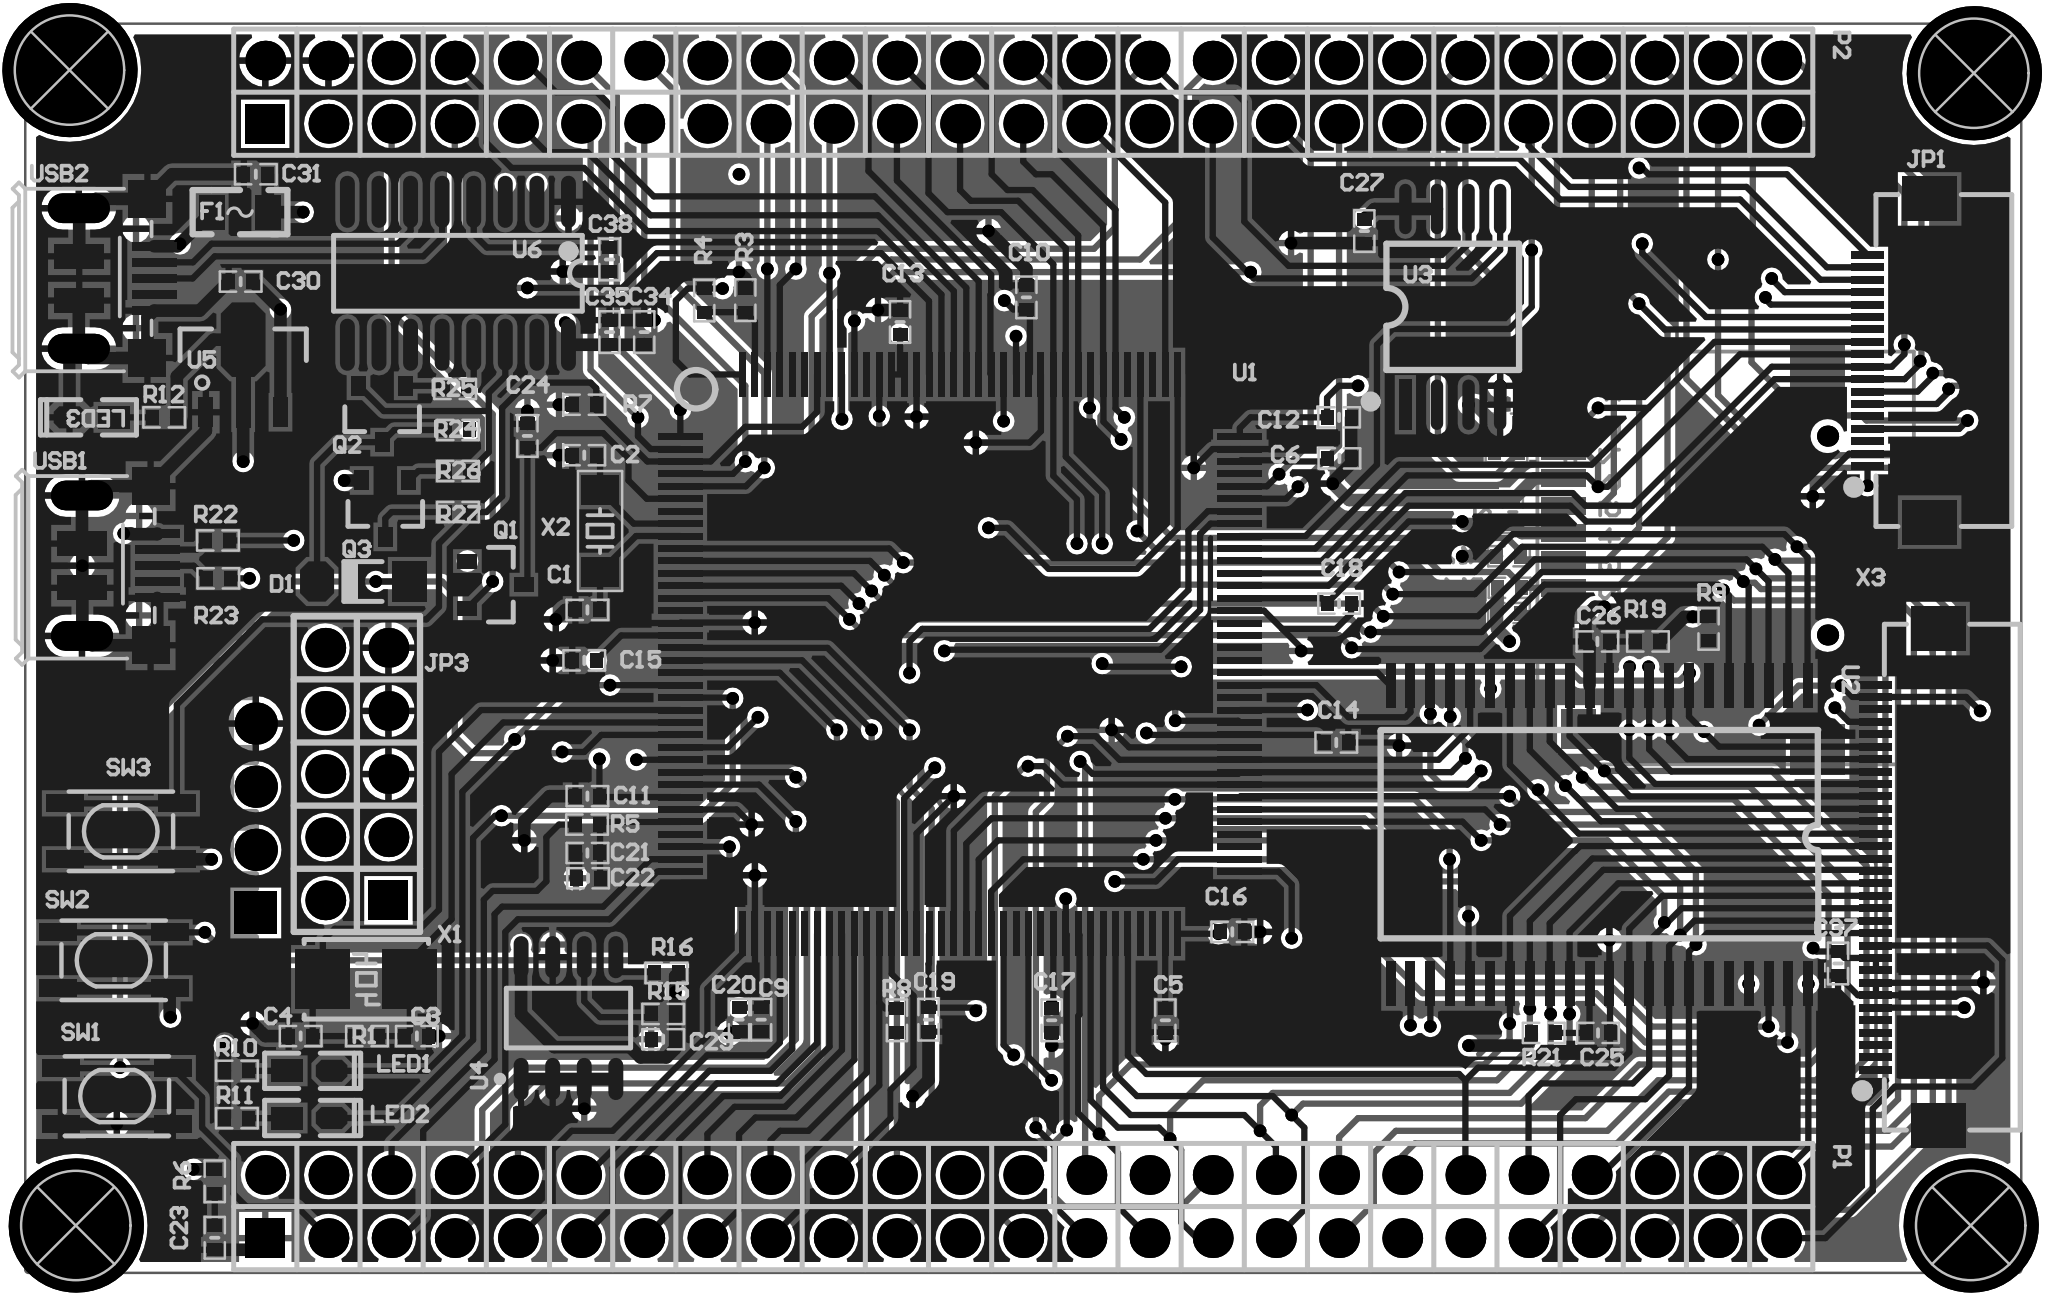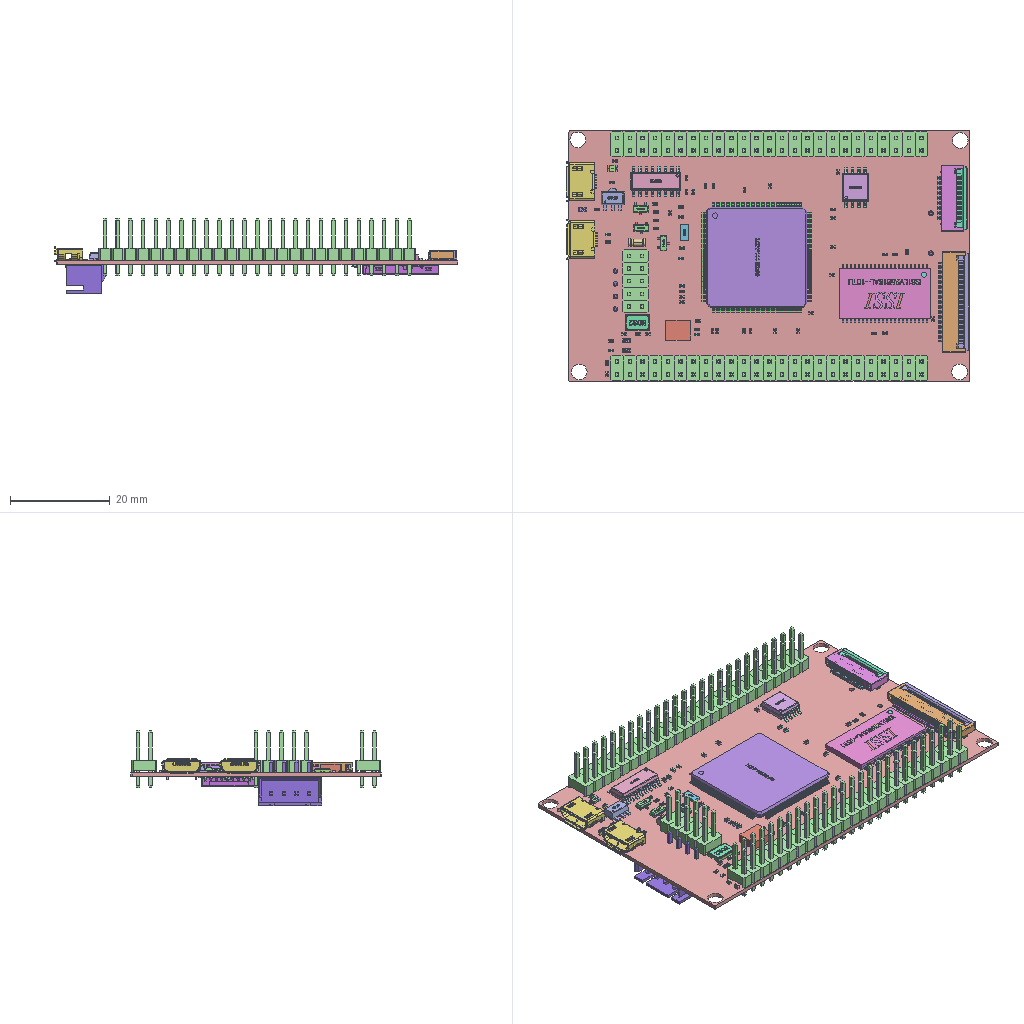Circuit board layout | Altium Designer | box 80.8 x 50.3 x 15 mm
Layer stack:
# Altium Designer layer stack of  (unit mm; dielectric type: 0 none, 1 core, 2 prepreg, 3 surface material)
index,name,kind,layer,copper_thickness_mm,dielectric_type,dielectric_thickness_mm,dielectric_material,dielectric_constant
0,Top Paste,other,,,,,,
1,Top Overlay,other,,,,,,
2,Top Solder,dielectric,,,3,0.0102,Solder Resist,3.5
3,Top Layer,copper,Top Layer,0.0356,,,,
4,Dielectric 1,dielectric,,,1,0.254,FR-4,4.2
5,2,copper,2,0.036,,,,
6,Dielectric 4,dielectric,,,2,0.127,,4.2
7,VCC,copper,VCC,0.036,,,,
8,Dielectric 3,dielectric,,,1,0.254,,4.2
9,Bottom Layer,copper,Bottom Layer,0.0356,,,,
10,Bottom Solder,dielectric,,,3,0.0102,Solder Resist,3.5
11,Bottom Overlay,other,,,,,,
12,Bottom Paste,other,,,,,,
# drill layer pairs: low layer,high layer
drill_pair,Top Layer,Bottom Layer
Part placement:
Designator,Comment,Layer,Footprint,Center-X(mm),Center-Y(mm),Rotation
C1,10P,TopLayer,C_0402,47.879,51.943,0
C2,10P,TopLayer,C_0402,47.752,58.166,0
C3,22P,TopLayer,C_0402,41.021,34.798,180
C4,22P,TopLayer,C_0402,36.347,34.798,0
C5,225,TopLayer,C_0402,71.12,35.433,270
C6,225,TopLayer,C_0402,78.12,58.039,0
C9,104,TopLayer,C_0402,54.864,35.458,90
C10,104,TopLayer,C_0402,65.532,64.516,270
C11,104,TopLayer,C_0402,47.879,44.45,0
C12,104,TopLayer,C_0402,78.105,59.69,180
C13,104,TopLayer,C_0402,60.452,63.525,270
C14,104,TopLayer,C_0402,77.993,46.609,180
C15,104,TopLayer,C_0402,47.752,49.911,360
C16,104,TopLayer,C_0402,73.812,38.989,180
C17,104,TopLayer,C_0402,66.548,35.433,90
C18,104,TopLayer,C_0402,78.105,52.197,180
C19,104,TopLayer,C_0402,61.595,35.458,90
C20,104,TopLayer,C_0402,53.975,35.458,90
C21,10UF,TopLayer,C_0402,47.879,42.164,180
C22,104,TopLayer,C_0402,47.904,41.148,180
C23,104,TopLayer,C_0402,32.893,26.685,270
C24,104,TopLayer,C_0402,45.466,58.943,270
C25,10U,TopLayer,C_0402,88.519,34.925,360
C26,10U,TopLayer,C_0402,88.494,50.673,180
C27,104,TopLayer,C_0402,79.121,67.183,270
C28,104,BottomLayer,C_0402,85.09,55.88,270
C29,104,TopLayer,C_0402,50.927,34.671,360
C30,22UF,TopLayer,C_0402,33.934,65.151,360
C31,104,TopLayer,C_0402,34.544,69.469,360
C34,10UF,TopLayer,C_0402,50.165,63.119,90
C35,104,TopLayer,C_0402,48.768,63.119,90
C37,104,TopLayer,C_0402,98.171,37.719,90
C38,104,TopLayer,C_0402,48.768,66.04,90
D1,1N4148,TopLayer,MINI_MELF_(LL34),38.862,53.086,180
F1,MSMD200-8V 2A,TopLayer,FU_0805,33.909,67.945,0
HOLE1,M3,TopLayer,M3_5.4MM,103.505,27.178,0
HOLE2,M3,TopLayer,M3_5.4MM,27.305,27.178,0
HOLE3,M3,TopLayer,M3_5.4MM,27.051,73.66,0
HOLE4,M3,TopLayer,M3_5.4MM,103.632,73.533,0
J1,TF_Card,BottomLayer,Micro_SD,92.436,54.084,270
JP1,FPC0.5-18P,TopLayer,FPC0.5_2H-WS-18P,100.606,61.976,90
JP2,SWD,BottomLayer,XH2.54-WI-4P,34.544,43.561,90
JP3,Header 5X2,TopLayer,HDR2.54-LI-2x5P,38.608,45.339,90
LED1,Red,TopLayer,LED_0603R,36.703,33.401,360
LED2,Red,TopLayer,LED_0603R,36.703,31.503,360
LED3,Red,TopLayer,LED_0603R,27.94,59.69,180
P1,Header 25X2,TopLayer,HDR2.54-LI-2x25P,65.405,27.94,360
P2,Header 25X2,TopLayer,HDR2.54-LI-2x25P,65.405,72.771,360
Q1,BAT54C,TopLayer,SOT23-3L,44.187,52.959,270
Q2,SS8050,TopLayer,SOT23-3L,39.624,59.826,180
Q3,SS8550,TopLayer,SOT23-3L,39.751,56.016,180
R1,1M,TopLayer,R_0402,39.014,34.798,180
R3,0R,TopLayer,R_0402,54.229,64.404,90
R4,0R,TopLayer,R_0402,52.578,64.389,90
R5,10R,TopLayer,R_0402,47.864,43.307,0
R6,10K,TopLayer,R_0402,32.893,28.956,90
R7,10K,TopLayer,R_0402,47.752,60.198,0
R8,10K,TopLayer,R_0402,60.325,35.433,90
R9,10K,TopLayer,R_0402,92.964,51.181,90
R10,510,TopLayer,R_0402,33.782,33.401,180
R11,510,TopLayer,R_0402,33.782,31.496,180
R12,1K,TopLayer,R_0402,30.861,59.69,360
R13,47K,BottomLayer,R_0402,84.938,51.816,360
R14,47K,BottomLayer,R_0402,84.963,52.832,360
R15,4.7K,TopLayer,R_0402,50.927,35.687,360
R16,4.7K,TopLayer,R_0402,51.054,37.338,360
R17,47K,BottomLayer,R_0402,84.938,54.102,360
R18,47K,BottomLayer,R_0402,84.836,58.293,360
R19,2R,TopLayer,R_0402,90.526,50.673,180
R20,47K,BottomLayer,R_0402,84.836,59.436,360
R21,2R,TopLayer,R_0402,86.335,34.925,360
R22,10R,TopLayer,R_0402,33.02,54.737,360
R23,10R,TopLayer,R_0402,33.035,53.213,360
R24,10K,TopLayer,R_0402,42.672,59.182,180
R25,1K,TopLayer,R_0402,42.56,60.833,180
R26,1K,TopLayer,R_0402,42.672,57.531,180
R27,1K,TopLayer,R_0402,42.672,55.88,360
SW1,3x6x5,TopLayer,TSW_SMD-3*4*2.5,28.956,32.385,360
SW2,3x6x5,TopLayer,TSW_SMD-3*4*2.5,28.829,37.846,180
SW3,3x6x5,TopLayer,TSW_SMD-3*4*2.5,29.119,43.035,180
U1,STM32F407,TopLayer,LQFP144_20X20_M,62.865,50.165,270
U2,IS61LV51216,TopLayer,TSOP44_M,88.576,42.895,270
U3,W25Q128,TopLayer,SOP8W_L,82.677,64.135,90
U4,24C02C-E/ST,TopLayer,SOP8_L,47.117,35.523,90
U5,AS1117B,TopLayer,SOT89_L,34.036,61.355,0
U6,CH340G,TopLayer,SOP16,42.672,65.486,270
USB1,USB-DEVICE,TopLayer,USB-MICRO_B,29.067,53.721,270
USB2,USB-DEVICE,TopLayer,USB-MICRO_B,28.94,65.278,270
X1,8MHz,TopLayer,OSC_5032-2P,38.989,37.084,180
X2,32.768KHZ,TopLayer,OSC_3215-2P,48.387,55.118,270
X3,FPC0.5-32P,TopLayer,FPC0.5_2H-WS-32P,100.944,41.192,90
Pad and via stacks:
# Altium Designer via and pad stacks of  (unit mm). Each distinct definition once, with the count of objects using it.
# via: kind,start_layer,end_layer,hole_mm,diameter_mm,mode(0 simple;1 top-mid-bottom;2 full stack),diameter_per_layer,count,example_net
# pad: kind,layer,hole_mm,hole_type(0 round;1 square;2 slot),plating,top_size,top_shape(1 round;2 rect;3 octagon;9 rounded rect),mid_size,bottom_size,mode,footprint,size_per_layer,count,example
pad,Top Layer,0,0,plated,0.508x0.6,2,0.508x0.6,0.508x0.6,0,R 0402,,42,R27.2
pad,Top Layer,0,0,unplated,2.4x2.2,2,2.4x2.2,2.4x2.2,0,OSC 5032-2P,,2,X1.2
pad,Top Layer,0,0,plated,1.27x0.889,3,1.27x0.889,1.27x0.889,0,LED 0603R,,3,LED3.2
pad,Top Layer,0,0,plated,1.27x0.889,2,1.27x0.889,1.27x0.889,0,LED 0603R,,3,LED3.1
pad,Top Layer,0,0,plated,0.508x0.6,2,0.508x0.6,0.508x0.6,0,C 0402,,64,C38.2
pad,Top Layer,0,0,plated,1.62x1.37,2,1.62x1.37,1.62x1.37,0,MINI_MELF (LL34),,1,D1.1
pad,Top Layer,0,0,plated,1.62x1.37,3,1.62x1.37,1.62x1.37,0,MINI_MELF (LL34),,1,D1.2
pad,Top Layer,0,0,plated,1.016x1.397,2,1.016x1.397,1.016x1.397,0,FU 0805,,2,F1.1
pad,Top Layer,0,0,plated,0.6x0.8,2,0.6x0.8,0.6x0.8,0,SOT23-3L,,9,Q1.1
pad,Top Layer,0,0,plated,0.254x1.8,2,0.254x1.8,0.254x1.8,0,LQFP144 20X20_M,,144,U1.11
pad,Top Layer,0,0,plated,1.8x0.4,2,1.8x0.4,1.8x0.4,0,TSOP44_M,,44,U2.39
pad,Top Layer,0,0,plated,2.032x0.5,1,2.032x0.5,2.032x0.5,0,SOP8W_L,,7,U3.8
pad,Top Layer,0,0,plated,2.032x0.5,2,2.032x0.5,2.032x0.5,0,SOP8W_L,,1,U3.1
pad,Top Layer,0,0,plated,0.6x1.7,1,0.6x1.7,0.6x1.7,0,SOP8_L,,8,U4.5
pad,Top Layer,0,0,plated,1.8x3,3,1.8x3,1.8x3,0,SOT89_L,,1,U5.2
pad,Top Layer,0,0,plated,0.6x1.2,2,0.6x1.2,0.6x1.2,0,SOT89_L,,2,U5.3
pad,Top Layer,0,0,plated,0.6x2.1,2,0.6x2.1,0.6x2.1,0,SOT89_L,,1,U5.2
pad,Top Layer,0,0,plated,0.6x2.1,1,0.6x2.1,0.6x2.1,0,SOP16,,16,U6.9
pad,Top Layer,0,0,plated,0.35x1.8,2,0.35x1.8,0.35x1.8,0,USB-MICRO_B,,10,USB1.5
pad,Top Layer,0,0,plated,1x2,2,1x2,1x2,0,USB-MICRO_B,,4,USB1.5
pad,Top Layer,0,0,plated,1.5x1.5,2,1.5x1.5,1.5x1.5,0,USB-MICRO_B,,4,USB1.5
pad,Top Layer,0,0,plated,1.2x1.5,2,1.2x1.5,1.2x1.5,0,OSC 3215-2P,,2,X2.2
pad,Top Layer,0,0,plated,1.3x0.3,2,1.3x0.3,1.3x0.3,0,FPC0.5 2H-WS-32P,,32,X3.32
pad,Top Layer,0,0,plated,2.2x1.8,2,2.2x1.8,2.2x1.8,0,FPC0.5 2H-WS-32P,,2,X3.0
pad,Top Layer,0,0,plated,1.5x0.7,2,1.5x0.7,1.5x0.7,0,TSW SMD-3*4*2.5,,12,SW1.2
pad,Top Layer,0,0,plated,2.2x1.8,2,2.2x1.8,2.2x1.8,0,FPC0.5 2H-WS-18P,,2,JP1.0
pad,Top Layer,0,0,plated,1.3x0.3,2,1.3x0.3,1.3x0.3,0,FPC0.5 2H-WS-18P,,18,JP1.9
pad,Multi-Layer,1,0,unplated,0.85x0.85,1,0.85x0.85,0.85x0.85,0,Micro SD,,2,J1.0
pad,Multi-Layer,3.175,0,plated,5.4x5.4,1,5.4x5.4,5.4x5.4,0,M3 5.4MM,,4,HOLE1.0
pad,Multi-Layer,0.9,0,plated,1.6x1.6,1,1.6x1.6,1.6x1.6,0,HDR2.54-LI-2x5P,,9,JP3.10
pad,Multi-Layer,0.9,0,plated,1.6x1.6,2,1.6x1.6,1.6x1.6,0,HDR2.54-LI-2x5P,,1,JP3.1
pad,Multi-Layer,0.9,0,plated,1.6x1.6,2,1.6x1.6,1.6x1.6,0,HDR2.54-LI-2x25P,,2,P1.1
pad,Multi-Layer,0.9,0,plated,1.6x1.6,1,1.6x1.6,1.6x1.6,0,HDR2.54-LI-2x25P,,98,P1.2
pad,Multi-Layer,0.45,2,plated,2.5x1.2,1,2.5x1.2,2.5x1.2,0,USB-MICRO_B,,4,USB1.5
pad,Multi-Layer,0.6,0,unplated,0x0,1,0x0,0x0,0,USB-MICRO_B,,4,USB1.5
pad,Multi-Layer,0.9,0,plated,1.7x1.7,1,1.7x1.7,1.7x1.7,0,XH2.54-WI-4P,,3,JP2.4
pad,Multi-Layer,0.9,0,plated,1.7x1.7,2,1.7x1.7,1.7x1.7,0,XH2.54-WI-4P,,1,JP2.1
pad,Bottom Layer,0,0,plated,0.508x0.6,2,0.508x0.6,0.508x0.6,0,R 0402,,10,R17.2
pad,Bottom Layer,0,0,plated,0.508x0.6,2,0.508x0.6,0.508x0.6,0,C 0402,,2,C28.2
pad,Bottom Layer,0,0,plated,2.032x2.2,2,2.032x2.2,2.032x2.2,0,Micro SD,,2,J1.10
pad,Bottom Layer,0,0,plated,1.6x1.4,2,1.6x1.4,1.6x1.4,0,Micro SD,,1,J1.10
pad,Bottom Layer,0,0,plated,1.2x1.4,2,1.2x1.4,1.2x1.4,0,Micro SD,,1,J1.10
pad,Bottom Layer,0,0,plated,0.7x1.8,2,0.7x1.8,0.7x1.8,0,Micro SD,,9,J1.1
via,Top Layer,Bottom Layer,0.254,0.508,0,,216,GND
Copper pours:
name,layer,net,type(0 solid;1 hatched;2 none)
D,Top Layer,GND,0
D,Bottom Layer,GND,0
Design rules, without the lines most boards share:
# Altium Designer design rules of  (exported by Altium Designer, unit mm)
# columns: name | kind | enabled | priority | scope1 | scope2 | descriptor | typed fields (field=value)
Clearance | 0 | enabled | 1 | All | All | Clearance Constraint (Gap=7mil) (All),(All) | gap=0.1778
PlaneConnect | 6 | enabled | 1 | All | All | Power Plane Connect Rule(Relief Connect )(Expansion=20mil) (Conductor Width=10mil) (Air Gap=10mil) (Entries=4) (All) | relief_conductor_width=0.254 relief_entries=4 relief_expansion=0.508
PolygonConnect | 20 | enabled | 1 | All | All | Polygon Connect Rule(Relief Connect )(Conductor Width=10mil) (Relief Angle=90 Angle) (Entries=4) (Air Gap Width=10mil) (All),(All) | connect_style(0=relief,1=direct,2=none)=0 relief_conductor_width=0.254 relief_entries=4
Width | 2 | enabled | 1 | All | All | Width Constraint (Min=7mil) (Max=30mil) (Preferred=7mil) (All) |
RoutingVias | 11 | enabled | 1 | All | All | Routing Via (MinHoleWidth=28mil) (MaxHoleWidth=28mil) (PreferredHoleWidth=28mil) (MinWidth=50mil) (MaxWidth=50mil) (PreferedWidth=50mil) (All) | via_min_hole=0.7112 via_max_hole=0.7112 via_preferred_diameter=1.27 via_preferred_hole=0.7112
SolderMaskExpansion | 13 | enabled | 1 | All | All | Solder Mask Expansion (Expansion =4mil) (All) | expansion=0.1016
HoleSize | 42 | enabled | 1 | All | All | Hole Size Constraint (Min=1mil) (Max=99999mil) (All) |
DiffPairsRouting | 51 | enabled | 1 | All | All | Differential Pairs Uncoupled Length using the Gap Constraints (Min=10mil) (Max=10mil) (Prefered=10mil)  and Width Constraints (Min=15mil) (Max=15mil) (Prefered=15mil) (All) |
HoleToHoleClearance | 52 | enabled | 1 | All | All | Hole To Hole Clearance (Gap=10mil) (All),(All) | gap=0.254
MinimumSolderMaskSliver | 53 | enabled | 1 | All | All | Minimum Solder Mask Sliver (Gap=0mil) (All),(All) |
SilkToSolderMaskClearance | 54 | enabled | 1 | IsPad | All | Silk To Solder Mask (Clearance=0mil) (IsPad),(All) |
SilkToSilkClearance | 55 | enabled | 1 | All | All | Silk to Silk (Clearance=0mil) (All),(All) |
Classes set for this board:
# Altium Designer classes of  (member kind: 0 net, 1 component, 2 from-to, 3 pad, 4 layer, 5 differential pair, 6 design channel, 7 polygon, 8 structure, 9 xSignal)
# columns: class name | member kind | superclass | members
Sheet1 | 1 | no | C1; C2; C3; C4; C5; C6; C9; C10; C11; C12; C13; C14; C15; C16; C17; C18; C19; C20; C21; C22; C23; C24; JP1; JP2; P1; P2; Q1; R1; R3; R4; R5; R6; R7; R8; SW1; U1; X1; X2;
Sheet2 | 1 | no | C25; C26; C27; C28; C29; C30; C31; C34; C35; C37; C38; D1; F1; HOLE1; HOLE2; HOLE3; HOLE4; J1; JP3; LED1; LED2; LED3; Q2; Q3; R9; R10; R11; R12; R13; R14; R15; R16; R17; R18; R19; R20; R21; R22; R23; R24; R25; R26; R27; SW2; SW3; U2; U3; U4; U5; U6; USB1; USB2; X3;